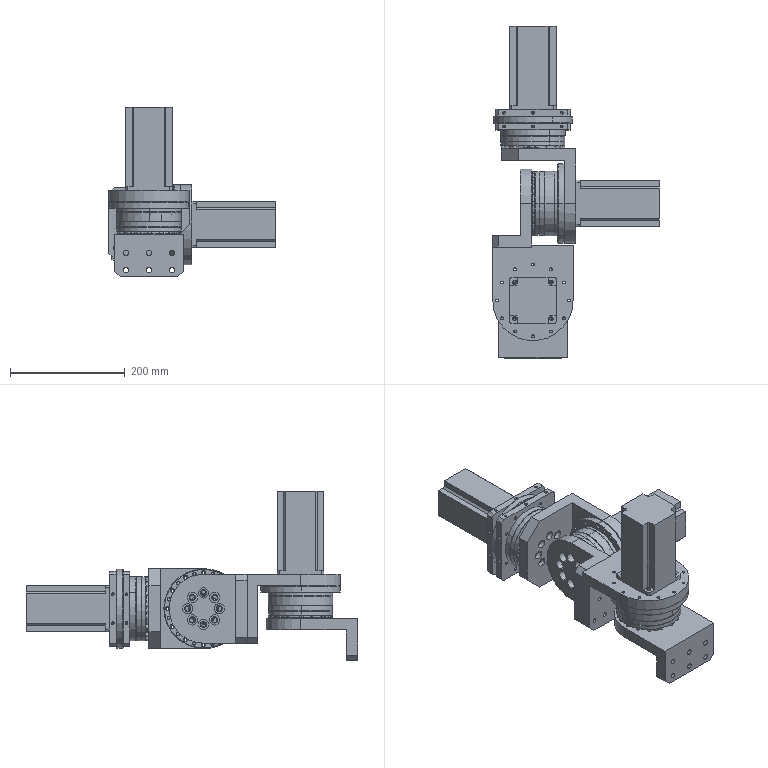Part | SolidWorks | features InContextFeatHolder 10 | 12 solids | 2921 faces | box 290 x 578 x 296 mm | volume 6218838 mm3 | cylinder 1510 | cone 752 | plane 611 | torus 48 | commonest cylinder face diameters 7 x208 5 x189 3.432 x144 4.5 x120 4.6 x96 5.188 x90